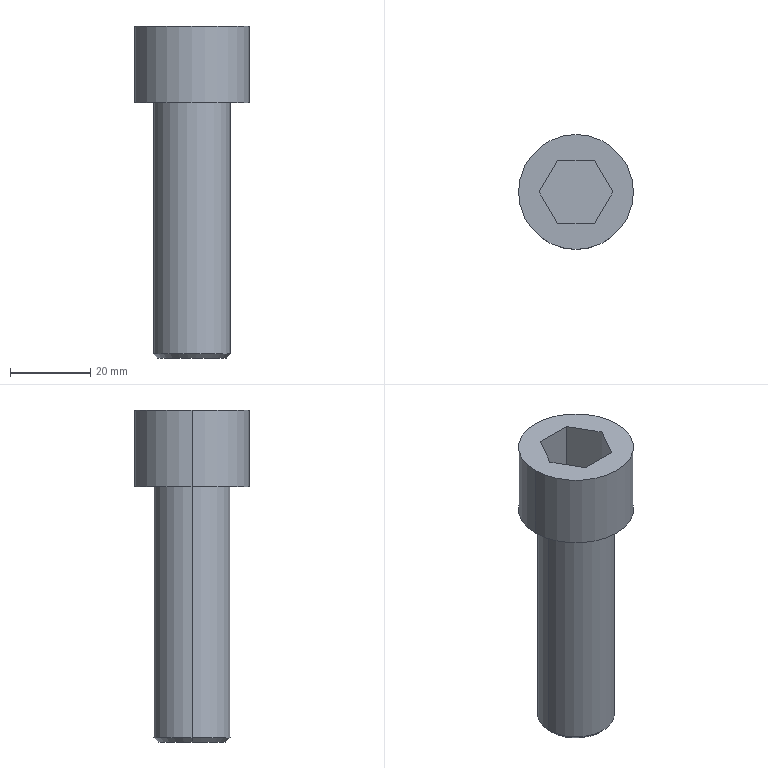Part | STEP file | 4-20.sldasm-Part-436 | 1 solid | 16 faces | box 28.575 x 28.575 x 82.55 mm | volume 27541 mm3 | plane 10 | cylinder 4 | cone 2 | commonest cylinder face diameters 19.05 x2 28.575 x2
STEP:
#1=CARTESIAN_POINT('',(176.506,150.,238.201));
#2=VERTEX_POINT('',#1);
#3=CARTESIAN_POINT('',(193.494,150.,238.201));
#4=VERTEX_POINT('',#3);
#5=CARTESIAN_POINT('',(185.,150.,238.201));
#6=DIRECTION('',(0.,0.,-1.));
#7=DIRECTION('',(1.,0.,0.));
#8=AXIS2_PLACEMENT_3D('',#5,#6,#7);
#9=CIRCLE('',#8,8.494);
#10=EDGE_CURVE('',#2,#4,#9,.T.);
#11=ORIENTED_EDGE('',*,*,#10,.F.);
#12=CARTESIAN_POINT('',(175.475,150.,239.232));
#13=VERTEX_POINT('',#12);
#14=CARTESIAN_POINT('',(175.475,150.,239.232));
#15=DIRECTION('',(-0.7071,0.,0.7071));
#16=VECTOR('',#15,1000.);
#17=LINE('',#14,#16);
#18=EDGE_CURVE('',#2,#13,#17,.T.);
#19=ORIENTED_EDGE('',*,*,#18,.T.);
#20=CARTESIAN_POINT('',(194.525,150.,239.232));
#21=VERTEX_POINT('',#20);
#22=CARTESIAN_POINT('',(185.,150.,239.232));
#23=DIRECTION('',(0.,0.,1.));
#24=DIRECTION('',(1.,0.,0.));
#25=AXIS2_PLACEMENT_3D('',#22,#23,#24);
#26=CIRCLE('',#25,9.525);
#27=EDGE_CURVE('',#21,#13,#26,.T.);
#28=ORIENTED_EDGE('',*,*,#27,.F.);
#29=CARTESIAN_POINT('',(194.525,150.,239.232));
#30=DIRECTION('',(0.7071,0.,0.7071));
#31=VECTOR('',#30,1000.);
#32=LINE('',#29,#31);
#33=EDGE_CURVE('',#4,#21,#32,.T.);
#34=ORIENTED_EDGE('',*,*,#33,.F.);
#35=EDGE_LOOP('',(#11,#19,#28,#34));
#36=FACE_OUTER_BOUND('',#35,.T.);
#37=CARTESIAN_POINT('',(185.,150.,239.232));
#38=DIRECTION('',(0.,0.,1.));
#39=DIRECTION('',(1.,0.,0.));
#40=AXIS2_PLACEMENT_3D('',#37,#38,#39);
#41=CONICAL_SURFACE('',#40,9.525,0.7854);
#42=ADVANCED_FACE('',(#36),#41,.T.);
#43=CARTESIAN_POINT('',(199.287,150.,301.701));
#44=VERTEX_POINT('',#43);
#45=CARTESIAN_POINT('',(170.712,150.,301.701));
#46=VERTEX_POINT('',#45);
#47=CARTESIAN_POINT('',(185.,150.,301.701));
#48=DIRECTION('',(0.,0.,1.));
#49=DIRECTION('',(1.,0.,0.));
#50=AXIS2_PLACEMENT_3D('',#47,#48,#49);
#51=CIRCLE('',#50,14.288);
#52=EDGE_CURVE('',#44,#46,#51,.T.);
#53=ORIENTED_EDGE('',*,*,#52,.T.);
#54=CARTESIAN_POINT('',(170.712,150.,320.751));
#55=VERTEX_POINT('',#54);
#56=CARTESIAN_POINT('',(170.712,150.,301.701));
#57=DIRECTION('',(0.,0.,1.));
#58=VECTOR('',#57,1000.);
#59=LINE('',#56,#58);
#60=EDGE_CURVE('',#46,#55,#59,.T.);
#61=ORIENTED_EDGE('',*,*,#60,.T.);
#62=CARTESIAN_POINT('',(199.287,150.,320.751));
#63=VERTEX_POINT('',#62);
#64=CARTESIAN_POINT('',(185.,150.,320.751));
#65=DIRECTION('',(0.,0.,1.));
#66=DIRECTION('',(1.,0.,0.));
#67=AXIS2_PLACEMENT_3D('',#64,#65,#66);
#68=CIRCLE('',#67,14.288);
#69=EDGE_CURVE('',#63,#55,#68,.T.);
#70=ORIENTED_EDGE('',*,*,#69,.F.);
#71=CARTESIAN_POINT('',(199.287,150.,301.701));
#72=DIRECTION('',(0.,0.,1.));
#73=VECTOR('',#72,1000.);
#74=LINE('',#71,#73);
#75=EDGE_CURVE('',#44,#63,#74,.T.);
#76=ORIENTED_EDGE('',*,*,#75,.F.);
#77=EDGE_LOOP('',(#53,#61,#70,#76));
#78=FACE_OUTER_BOUND('',#77,.T.);
#79=CARTESIAN_POINT('',(185.,150.,301.701));
#80=DIRECTION('',(0.,0.,1.));
#81=DIRECTION('',(1.,0.,0.));
#82=AXIS2_PLACEMENT_3D('',#79,#80,#81);
#83=CYLINDRICAL_SURFACE('',#82,14.288);
#84=ADVANCED_FACE('',(#78),#83,.T.);
#85=CARTESIAN_POINT('',(194.525,150.,301.701));
#86=VERTEX_POINT('',#85);
#87=CARTESIAN_POINT('',(175.475,150.,301.701));
#88=VERTEX_POINT('',#87);
#89=CARTESIAN_POINT('',(185.,150.,301.701));
#90=DIRECTION('',(0.,0.,1.));
#91=DIRECTION('',(1.,0.,0.));
#92=AXIS2_PLACEMENT_3D('',#89,#90,#91);
#93=CIRCLE('',#92,9.525);
#94=EDGE_CURVE('',#86,#88,#93,.T.);
#95=ORIENTED_EDGE('',*,*,#94,.F.);
#96=CARTESIAN_POINT('',(194.525,150.,301.701));
#97=DIRECTION('',(0.,0.,-1.));
#98=VECTOR('',#97,1000.);
#99=LINE('',#96,#98);
#100=EDGE_CURVE('',#86,#21,#99,.T.);
#101=ORIENTED_EDGE('',*,*,#100,.T.);
#102=ORIENTED_EDGE('',*,*,#27,.T.);
#103=CARTESIAN_POINT('',(175.475,150.,301.701));
#104=DIRECTION('',(0.,0.,-1.));
#105=VECTOR('',#104,1000.);
#106=LINE('',#103,#105);
#107=EDGE_CURVE('',#88,#13,#106,.T.);
#108=ORIENTED_EDGE('',*,*,#107,.F.);
#109=EDGE_LOOP('',(#95,#101,#102,#108));
#110=FACE_OUTER_BOUND('',#109,.T.);
#111=CARTESIAN_POINT('',(185.,150.,301.701));
#112=DIRECTION('',(0.,0.,-1.));
#113=DIRECTION('',(-1.,0.,0.));
#114=AXIS2_PLACEMENT_3D('',#111,#112,#113);
#115=CYLINDRICAL_SURFACE('',#114,9.525);
#116=ADVANCED_FACE('',(#110),#115,.T.);
#117=ORIENTED_EDGE('',*,*,#100,.F.);
#118=CARTESIAN_POINT('',(185.,150.,301.701));
#119=DIRECTION('',(0.,0.,1.));
#120=DIRECTION('',(1.,0.,0.));
#121=AXIS2_PLACEMENT_3D('',#118,#119,#120);
#122=CIRCLE('',#121,9.525);
#123=EDGE_CURVE('',#88,#86,#122,.T.);
#124=ORIENTED_EDGE('',*,*,#123,.F.);
#125=ORIENTED_EDGE('',*,*,#107,.T.);
#126=CARTESIAN_POINT('',(185.,150.,239.232));
#127=DIRECTION('',(0.,0.,1.));
#128=DIRECTION('',(1.,0.,0.));
#129=AXIS2_PLACEMENT_3D('',#126,#127,#128);
#130=CIRCLE('',#129,9.525);
#131=EDGE_CURVE('',#13,#21,#130,.T.);
#132=ORIENTED_EDGE('',*,*,#131,.T.);
#133=EDGE_LOOP('',(#117,#124,#125,#132));
#134=FACE_OUTER_BOUND('',#133,.T.);
#135=CARTESIAN_POINT('',(185.,150.,301.701));
#136=DIRECTION('',(0.,0.,-1.));
#137=DIRECTION('',(-1.,0.,0.));
#138=AXIS2_PLACEMENT_3D('',#135,#136,#137);
#139=CYLINDRICAL_SURFACE('',#138,9.525);
#140=ADVANCED_FACE('',(#134),#139,.T.);
#141=CARTESIAN_POINT('',(185.,150.,238.201));
#142=DIRECTION('',(0.,0.,-1.));
#143=DIRECTION('',(1.,0.,0.));
#144=AXIS2_PLACEMENT_3D('',#141,#142,#143);
#145=CIRCLE('',#144,8.494);
#146=EDGE_CURVE('',#4,#2,#145,.T.);
#147=ORIENTED_EDGE('',*,*,#146,.T.);
#148=ORIENTED_EDGE('',*,*,#10,.T.);
#149=EDGE_LOOP('',(#147,#148));
#150=FACE_OUTER_BOUND('',#149,.T.);
#151=CARTESIAN_POINT('',(185.,150.,238.201));
#152=DIRECTION('',(0.,0.,1.));
#153=DIRECTION('',(1.,0.,0.));
#154=AXIS2_PLACEMENT_3D('',#151,#152,#153);
#155=PLANE('',#154);
#156=ADVANCED_FACE('',(#150),#155,.F.);
#157=ORIENTED_EDGE('',*,*,#52,.F.);
#158=CARTESIAN_POINT('',(185.,150.,301.701));
#159=DIRECTION('',(0.,0.,1.));
#160=DIRECTION('',(1.,0.,0.));
#161=AXIS2_PLACEMENT_3D('',#158,#159,#160);
#162=CIRCLE('',#161,14.288);
#163=EDGE_CURVE('',#46,#44,#162,.T.);
#164=ORIENTED_EDGE('',*,*,#163,.F.);
#165=EDGE_LOOP('',(#157,#164));
#166=FACE_OUTER_BOUND('',#165,.T.);
#167=ORIENTED_EDGE('',*,*,#123,.T.);
#168=ORIENTED_EDGE('',*,*,#94,.T.);
#169=EDGE_LOOP('',(#167,#168));
#170=FACE_BOUND('',#169,.T.);
#171=CARTESIAN_POINT('',(185.,150.,301.701));
#172=DIRECTION('',(0.,0.,-1.));
#173=DIRECTION('',(-1.,0.,0.));
#174=AXIS2_PLACEMENT_3D('',#171,#172,#173);
#175=PLANE('',#174);
#176=ADVANCED_FACE('',(#166,#170),#175,.T.);
#177=CARTESIAN_POINT('',(180.417,142.062,320.751));
#178=VERTEX_POINT('',#177);
#179=CARTESIAN_POINT('',(189.583,142.062,320.751));
#180=VERTEX_POINT('',#179);
#181=CARTESIAN_POINT('',(180.417,142.062,320.751));
#182=DIRECTION('',(1.,0.,0.));
#183=VECTOR('',#182,1000.);
#184=LINE('',#181,#183);
#185=EDGE_CURVE('',#178,#180,#184,.T.);
#186=ORIENTED_EDGE('',*,*,#185,.F.);
#187=CARTESIAN_POINT('',(175.835,150.,320.751));
#188=VERTEX_POINT('',#187);
#189=CARTESIAN_POINT('',(175.835,150.,320.751));
#190=DIRECTION('',(0.5,-0.866,0.));
#191=VECTOR('',#190,1000.);
#192=LINE('',#189,#191);
#193=EDGE_CURVE('',#188,#178,#192,.T.);
#194=ORIENTED_EDGE('',*,*,#193,.F.);
#195=CARTESIAN_POINT('',(180.417,157.938,320.751));
#196=VERTEX_POINT('',#195);
#197=CARTESIAN_POINT('',(180.417,157.938,320.751));
#198=DIRECTION('',(-0.5,-0.866,0.));
#199=VECTOR('',#198,1000.);
#200=LINE('',#197,#199);
#201=EDGE_CURVE('',#196,#188,#200,.T.);
#202=ORIENTED_EDGE('',*,*,#201,.F.);
#203=CARTESIAN_POINT('',(189.583,157.938,320.751));
#204=VERTEX_POINT('',#203);
#205=CARTESIAN_POINT('',(189.583,157.938,320.751));
#206=DIRECTION('',(-1.,0.,0.));
#207=VECTOR('',#206,1000.);
#208=LINE('',#205,#207);
#209=EDGE_CURVE('',#204,#196,#208,.T.);
#210=ORIENTED_EDGE('',*,*,#209,.F.);
#211=CARTESIAN_POINT('',(194.165,150.,320.751));
#212=VERTEX_POINT('',#211);
#213=CARTESIAN_POINT('',(194.165,150.,320.751));
#214=DIRECTION('',(-0.5,0.866,0.));
#215=VECTOR('',#214,1000.);
#216=LINE('',#213,#215);
#217=EDGE_CURVE('',#212,#204,#216,.T.);
#218=ORIENTED_EDGE('',*,*,#217,.F.);
#219=CARTESIAN_POINT('',(189.583,142.062,320.751));
#220=DIRECTION('',(0.5,0.866,0.));
#221=VECTOR('',#220,1000.);
#222=LINE('',#219,#221);
#223=EDGE_CURVE('',#180,#212,#222,.T.);
#224=ORIENTED_EDGE('',*,*,#223,.F.);
#225=EDGE_LOOP('',(#186,#194,#202,#210,#218,#224));
#226=FACE_BOUND('',#225,.T.);
#227=ORIENTED_EDGE('',*,*,#69,.T.);
#228=CARTESIAN_POINT('',(185.,150.,320.751));
#229=DIRECTION('',(0.,0.,1.));
#230=DIRECTION('',(1.,0.,0.));
#231=AXIS2_PLACEMENT_3D('',#228,#229,#230);
#232=CIRCLE('',#231,14.288);
#233=EDGE_CURVE('',#55,#63,#232,.T.);
#234=ORIENTED_EDGE('',*,*,#233,.T.);
#235=EDGE_LOOP('',(#227,#234));
#236=FACE_OUTER_BOUND('',#235,.T.);
#237=CARTESIAN_POINT('',(185.,150.,320.751));
#238=DIRECTION('',(0.,0.,1.));
#239=DIRECTION('',(1.,0.,0.));
#240=AXIS2_PLACEMENT_3D('',#237,#238,#239);
#241=PLANE('',#240);
#242=ADVANCED_FACE('',(#226,#236),#241,.T.);
#243=ORIENTED_EDGE('',*,*,#60,.F.);
#244=ORIENTED_EDGE('',*,*,#163,.T.);
#245=ORIENTED_EDGE('',*,*,#75,.T.);
#246=ORIENTED_EDGE('',*,*,#233,.F.);
#247=EDGE_LOOP('',(#243,#244,#245,#246));
#248=FACE_OUTER_BOUND('',#247,.T.);
#249=CARTESIAN_POINT('',(185.,150.,301.701));
#250=DIRECTION('',(0.,0.,1.));
#251=DIRECTION('',(1.,0.,0.));
#252=AXIS2_PLACEMENT_3D('',#249,#250,#251);
#253=CYLINDRICAL_SURFACE('',#252,14.288);
#254=ADVANCED_FACE('',(#248),#253,.T.);
#255=ORIENTED_EDGE('',*,*,#18,.F.);
#256=ORIENTED_EDGE('',*,*,#146,.F.);
#257=ORIENTED_EDGE('',*,*,#33,.T.);
#258=ORIENTED_EDGE('',*,*,#131,.F.);
#259=EDGE_LOOP('',(#255,#256,#257,#258));
#260=FACE_OUTER_BOUND('',#259,.T.);
#261=CARTESIAN_POINT('',(185.,150.,239.232));
#262=DIRECTION('',(0.,0.,1.));
#263=DIRECTION('',(1.,0.,0.));
#264=AXIS2_PLACEMENT_3D('',#261,#262,#263);
#265=CONICAL_SURFACE('',#264,9.525,0.7854);
#266=ADVANCED_FACE('',(#260),#265,.T.);
#267=ORIENTED_EDGE('',*,*,#185,.T.);
#268=CARTESIAN_POINT('',(189.583,142.062,308.178));
#269=VERTEX_POINT('',#268);
#270=CARTESIAN_POINT('',(189.583,142.062,308.178));
#271=DIRECTION('',(0.,0.,1.));
#272=VECTOR('',#271,1000.);
#273=LINE('',#270,#272);
#274=EDGE_CURVE('',#269,#180,#273,.T.);
#275=ORIENTED_EDGE('',*,*,#274,.F.);
#276=CARTESIAN_POINT('',(180.417,142.062,308.178));
#277=VERTEX_POINT('',#276);
#278=CARTESIAN_POINT('',(180.417,142.062,308.178));
#279=DIRECTION('',(1.,0.,0.));
#280=VECTOR('',#279,1000.);
#281=LINE('',#278,#280);
#282=EDGE_CURVE('',#277,#269,#281,.T.);
#283=ORIENTED_EDGE('',*,*,#282,.F.);
#284=CARTESIAN_POINT('',(180.417,142.062,308.178));
#285=DIRECTION('',(0.,0.,1.));
#286=VECTOR('',#285,1000.);
#287=LINE('',#284,#286);
#288=EDGE_CURVE('',#277,#178,#287,.T.);
#289=ORIENTED_EDGE('',*,*,#288,.T.);
#290=EDGE_LOOP('',(#267,#275,#283,#289));
#291=FACE_OUTER_BOUND('',#290,.T.);
#292=CARTESIAN_POINT('',(180.417,142.062,308.178));
#293=DIRECTION('',(0.,-1.,0.));
#294=DIRECTION('',(0.,0.,-1.));
#295=AXIS2_PLACEMENT_3D('',#292,#293,#294);
#296=PLANE('',#295);
#297=ADVANCED_FACE('',(#291),#296,.F.);
#298=ORIENTED_EDGE('',*,*,#223,.T.);
#299=CARTESIAN_POINT('',(194.165,150.,308.178));
#300=VERTEX_POINT('',#299);
#301=CARTESIAN_POINT('',(194.165,150.,308.178));
#302=DIRECTION('',(0.,0.,1.));
#303=VECTOR('',#302,1000.);
#304=LINE('',#301,#303);
#305=EDGE_CURVE('',#300,#212,#304,.T.);
#306=ORIENTED_EDGE('',*,*,#305,.F.);
#307=CARTESIAN_POINT('',(189.583,142.062,308.178));
#308=DIRECTION('',(0.5,0.866,0.));
#309=VECTOR('',#308,1000.);
#310=LINE('',#307,#309);
#311=EDGE_CURVE('',#269,#300,#310,.T.);
#312=ORIENTED_EDGE('',*,*,#311,.F.);
#313=ORIENTED_EDGE('',*,*,#274,.T.);
#314=EDGE_LOOP('',(#298,#306,#312,#313));
#315=FACE_OUTER_BOUND('',#314,.T.);
#316=CARTESIAN_POINT('',(189.583,142.062,308.178));
#317=DIRECTION('',(0.866,-0.5,0.));
#318=DIRECTION('',(0.5,0.866,0.));
#319=AXIS2_PLACEMENT_3D('',#316,#317,#318);
#320=PLANE('',#319);
#321=ADVANCED_FACE('',(#315),#320,.F.);
#322=ORIENTED_EDGE('',*,*,#217,.T.);
#323=CARTESIAN_POINT('',(189.583,157.938,308.178));
#324=VERTEX_POINT('',#323);
#325=CARTESIAN_POINT('',(189.583,157.938,308.178));
#326=DIRECTION('',(0.,0.,1.));
#327=VECTOR('',#326,1000.);
#328=LINE('',#325,#327);
#329=EDGE_CURVE('',#324,#204,#328,.T.);
#330=ORIENTED_EDGE('',*,*,#329,.F.);
#331=CARTESIAN_POINT('',(194.165,150.,308.178));
#332=DIRECTION('',(-0.5,0.866,0.));
#333=VECTOR('',#332,1000.);
#334=LINE('',#331,#333);
#335=EDGE_CURVE('',#300,#324,#334,.T.);
#336=ORIENTED_EDGE('',*,*,#335,.F.);
#337=ORIENTED_EDGE('',*,*,#305,.T.);
#338=EDGE_LOOP('',(#322,#330,#336,#337));
#339=FACE_OUTER_BOUND('',#338,.T.);
#340=CARTESIAN_POINT('',(194.165,150.,308.178));
#341=DIRECTION('',(0.866,0.5,0.));
#342=DIRECTION('',(-0.5,0.866,0.));
#343=AXIS2_PLACEMENT_3D('',#340,#341,#342);
#344=PLANE('',#343);
#345=ADVANCED_FACE('',(#339),#344,.F.);
#346=ORIENTED_EDGE('',*,*,#209,.T.);
#347=CARTESIAN_POINT('',(180.417,157.938,308.178));
#348=VERTEX_POINT('',#347);
#349=CARTESIAN_POINT('',(180.417,157.938,308.178));
#350=DIRECTION('',(0.,0.,1.));
#351=VECTOR('',#350,1000.);
#352=LINE('',#349,#351);
#353=EDGE_CURVE('',#348,#196,#352,.T.);
#354=ORIENTED_EDGE('',*,*,#353,.F.);
#355=CARTESIAN_POINT('',(189.583,157.938,308.178));
#356=DIRECTION('',(-1.,0.,0.));
#357=VECTOR('',#356,1000.);
#358=LINE('',#355,#357);
#359=EDGE_CURVE('',#324,#348,#358,.T.);
#360=ORIENTED_EDGE('',*,*,#359,.F.);
#361=ORIENTED_EDGE('',*,*,#329,.T.);
#362=EDGE_LOOP('',(#346,#354,#360,#361));
#363=FACE_OUTER_BOUND('',#362,.T.);
#364=CARTESIAN_POINT('',(189.583,157.938,308.178));
#365=DIRECTION('',(0.,1.,0.));
#366=DIRECTION('',(0.,0.,1.));
#367=AXIS2_PLACEMENT_3D('',#364,#365,#366);
#368=PLANE('',#367);
#369=ADVANCED_FACE('',(#363),#368,.F.);
#370=ORIENTED_EDGE('',*,*,#201,.T.);
#371=CARTESIAN_POINT('',(175.835,150.,308.178));
#372=VERTEX_POINT('',#371);
#373=CARTESIAN_POINT('',(175.835,150.,308.178));
#374=DIRECTION('',(0.,0.,1.));
#375=VECTOR('',#374,1000.);
#376=LINE('',#373,#375);
#377=EDGE_CURVE('',#372,#188,#376,.T.);
#378=ORIENTED_EDGE('',*,*,#377,.F.);
#379=CARTESIAN_POINT('',(180.417,157.938,308.178));
#380=DIRECTION('',(-0.5,-0.866,0.));
#381=VECTOR('',#380,1000.);
#382=LINE('',#379,#381);
#383=EDGE_CURVE('',#348,#372,#382,.T.);
#384=ORIENTED_EDGE('',*,*,#383,.F.);
#385=ORIENTED_EDGE('',*,*,#353,.T.);
#386=EDGE_LOOP('',(#370,#378,#384,#385));
#387=FACE_OUTER_BOUND('',#386,.T.);
#388=CARTESIAN_POINT('',(180.417,157.938,308.178));
#389=DIRECTION('',(-0.866,0.5,0.));
#390=DIRECTION('',(-0.5,-0.866,0.));
#391=AXIS2_PLACEMENT_3D('',#388,#389,#390);
#392=PLANE('',#391);
#393=ADVANCED_FACE('',(#387),#392,.F.);
#394=ORIENTED_EDGE('',*,*,#193,.T.);
#395=ORIENTED_EDGE('',*,*,#288,.F.);
#396=CARTESIAN_POINT('',(175.835,150.,308.178));
#397=DIRECTION('',(0.5,-0.866,0.));
#398=VECTOR('',#397,1000.);
#399=LINE('',#396,#398);
#400=EDGE_CURVE('',#372,#277,#399,.T.);
#401=ORIENTED_EDGE('',*,*,#400,.F.);
#402=ORIENTED_EDGE('',*,*,#377,.T.);
#403=EDGE_LOOP('',(#394,#395,#401,#402));
#404=FACE_OUTER_BOUND('',#403,.T.);
#405=CARTESIAN_POINT('',(175.835,150.,308.178));
#406=DIRECTION('',(-0.866,-0.5,0.));
#407=DIRECTION('',(0.5,-0.866,0.));
#408=AXIS2_PLACEMENT_3D('',#405,#406,#407);
#409=PLANE('',#408);
#410=ADVANCED_FACE('',(#404),#409,.F.);
#411=ORIENTED_EDGE('',*,*,#282,.T.);
#412=ORIENTED_EDGE('',*,*,#311,.T.);
#413=ORIENTED_EDGE('',*,*,#335,.T.);
#414=ORIENTED_EDGE('',*,*,#359,.T.);
#415=ORIENTED_EDGE('',*,*,#383,.T.);
#416=ORIENTED_EDGE('',*,*,#400,.T.);
#417=EDGE_LOOP('',(#411,#412,#413,#414,#415,#416));
#418=FACE_OUTER_BOUND('',#417,.T.);
#419=CARTESIAN_POINT('',(189.583,142.062,308.178));
#420=DIRECTION('',(0.,0.,1.));
#421=DIRECTION('',(1.,0.,0.));
#422=AXIS2_PLACEMENT_3D('',#419,#420,#421);
#423=PLANE('',#422);
#424=ADVANCED_FACE('',(#418),#423,.T.);
#425=CLOSED_SHELL('',(#42,#84,#116,#140,#156,#176,#242,#254,#266,#297,#321,#345,#369,#393,#410,#424));
#426=MANIFOLD_SOLID_BREP('',#425);
#427=CARTESIAN_POINT('',(0.,0.,0.));
#428=DIRECTION('',(0.,0.,1.));
#429=DIRECTION('',(1.,0.,0.));
#430=AXIS2_PLACEMENT_3D('',#427,#428,#429);
#431=(LENGTH_UNIT()NAMED_UNIT(*)SI_UNIT(.MILLI.,.METRE.));
#432=UNCERTAINTY_MEASURE_WITH_UNIT(LENGTH_MEASURE(0.00001),#431,'','');
#433=(NAMED_UNIT(*)PLANE_ANGLE_UNIT()SI_UNIT($,.RADIAN.));
#434=(NAMED_UNIT(*)SI_UNIT($,.STERADIAN.)SOLID_ANGLE_UNIT());
#435=(GEOMETRIC_REPRESENTATION_CONTEXT(3)GLOBAL_UNCERTAINTY_ASSIGNED_CONTEXT((#432))GLOBAL_UNIT_ASSIGNED_CONTEXT((#431,#433,#434))REPRESENTATION_CONTEXT('',''));
#436=ADVANCED_BREP_SHAPE_REPRESENTATION('',(#426,#430),#435);